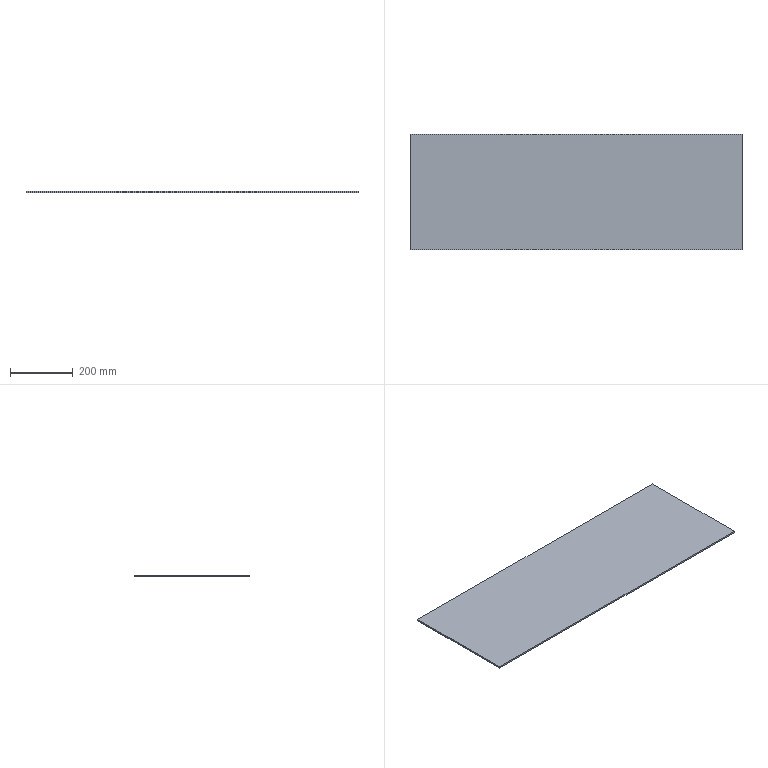Part | STEP file | JZHM | 1 solid | 6 faces | box 1060 x 370 x 5 mm | volume 1961000 mm3 | plane 6
STEP:
#1=CARTESIAN_POINT('',(0.,0.,0.));
#2=DIRECTION('',(0.,0.,1.));
#3=DIRECTION('',(1.,0.,0.));
#4=AXIS2_PLACEMENT_3D('',#1,#2,#3);
#5=CARTESIAN_POINT('',(-530.,185.,0.));
#6=VERTEX_POINT('',#5);
#7=CARTESIAN_POINT('',(-530.,-185.,0.));
#8=VERTEX_POINT('',#7);
#9=CARTESIAN_POINT('',(-530.,185.,0.));
#10=DIRECTION('',(0.,-1.,0.));
#11=VECTOR('',#10,1.);
#12=LINE('',#9,#11);
#13=CARTESIAN_POINT('',(-530.,185.,5.));
#14=DIRECTION('',(1.,0.,0.));
#15=DIRECTION('',(0.,0.,-1.));
#16=AXIS2_PLACEMENT_3D('',#13,#14,#15);
#17=PLANE('',#16);
#18=CARTESIAN_POINT('',(5.,0.));
#19=DIRECTION('',(0.,-1.));
#20=VECTOR('',#19,1.);
#21=LINE('',#18,#20);
#22=(GEOMETRIC_REPRESENTATION_CONTEXT(2)PARAMETRIC_REPRESENTATION_CONTEXT()REPRESENTATION_CONTEXT('',''));
#23=DEFINITIONAL_REPRESENTATION('',(#21),#22);
#24=PCURVE('',#17,#23);
#25=CARTESIAN_POINT('',(-530.,-185.,0.));
#26=DIRECTION('',(0.,0.,1.));
#27=DIRECTION('',(1.,0.,0.));
#28=AXIS2_PLACEMENT_3D('',#25,#26,#27);
#29=PLANE('',#28);
#30=CARTESIAN_POINT('',(0.,370.));
#31=DIRECTION('',(0.,-1.));
#32=VECTOR('',#31,1.);
#33=LINE('',#30,#32);
#34=(GEOMETRIC_REPRESENTATION_CONTEXT(2)PARAMETRIC_REPRESENTATION_CONTEXT()REPRESENTATION_CONTEXT('',''));
#35=DEFINITIONAL_REPRESENTATION('',(#33),#34);
#36=PCURVE('',#29,#35);
#37=SURFACE_CURVE('',#12,(#24,#36),.PCURVE_S1.);
#38=EDGE_CURVE('',#6,#8,#37,.T.);
#39=ORIENTED_EDGE('',*,*,#38,.T.);
#40=CARTESIAN_POINT('',(-530.,-185.,5.));
#41=VERTEX_POINT('',#40);
#42=CARTESIAN_POINT('',(-530.,-185.,5.));
#43=DIRECTION('',(0.,0.,-1.));
#44=VECTOR('',#43,1.);
#45=LINE('',#42,#44);
#46=CARTESIAN_POINT('',(0.,-370.));
#47=DIRECTION('',(1.,0.));
#48=VECTOR('',#47,1.);
#49=LINE('',#46,#48);
#50=(GEOMETRIC_REPRESENTATION_CONTEXT(2)PARAMETRIC_REPRESENTATION_CONTEXT()REPRESENTATION_CONTEXT('',''));
#51=DEFINITIONAL_REPRESENTATION('',(#49),#50);
#52=PCURVE('',#17,#51);
#53=CARTESIAN_POINT('',(-530.,-185.,5.));
#54=DIRECTION('',(0.,1.,0.));
#55=DIRECTION('',(0.,0.,1.));
#56=AXIS2_PLACEMENT_3D('',#53,#54,#55);
#57=PLANE('',#56);
#58=CARTESIAN_POINT('',(0.,0.));
#59=DIRECTION('',(-1.,0.));
#60=VECTOR('',#59,1.);
#61=LINE('',#58,#60);
#62=(GEOMETRIC_REPRESENTATION_CONTEXT(2)PARAMETRIC_REPRESENTATION_CONTEXT()REPRESENTATION_CONTEXT('',''));
#63=DEFINITIONAL_REPRESENTATION('',(#61),#62);
#64=PCURVE('',#57,#63);
#65=SURFACE_CURVE('',#45,(#52,#64),.PCURVE_S1.);
#66=EDGE_CURVE('',#41,#8,#65,.T.);
#67=ORIENTED_EDGE('',*,*,#66,.F.);
#68=CARTESIAN_POINT('',(-530.,185.,5.));
#69=VERTEX_POINT('',#68);
#70=CARTESIAN_POINT('',(-530.,185.,5.));
#71=DIRECTION('',(0.,-1.,0.));
#72=VECTOR('',#71,1.);
#73=LINE('',#70,#72);
#74=CARTESIAN_POINT('',(0.,0.));
#75=DIRECTION('',(0.,-1.));
#76=VECTOR('',#75,1.);
#77=LINE('',#74,#76);
#78=(GEOMETRIC_REPRESENTATION_CONTEXT(2)PARAMETRIC_REPRESENTATION_CONTEXT()REPRESENTATION_CONTEXT('',''));
#79=DEFINITIONAL_REPRESENTATION('',(#77),#78);
#80=PCURVE('',#17,#79);
#81=CARTESIAN_POINT('',(-530.,-185.,5.));
#82=DIRECTION('',(0.,0.,1.));
#83=DIRECTION('',(1.,0.,0.));
#84=AXIS2_PLACEMENT_3D('',#81,#82,#83);
#85=PLANE('',#84);
#86=CARTESIAN_POINT('',(0.,370.));
#87=DIRECTION('',(0.,-1.));
#88=VECTOR('',#87,1.);
#89=LINE('',#86,#88);
#90=(GEOMETRIC_REPRESENTATION_CONTEXT(2)PARAMETRIC_REPRESENTATION_CONTEXT()REPRESENTATION_CONTEXT('',''));
#91=DEFINITIONAL_REPRESENTATION('',(#89),#90);
#92=PCURVE('',#85,#91);
#93=SURFACE_CURVE('',#73,(#80,#92),.PCURVE_S1.);
#94=EDGE_CURVE('',#69,#41,#93,.T.);
#95=ORIENTED_EDGE('',*,*,#94,.F.);
#96=CARTESIAN_POINT('',(-530.,185.,5.));
#97=DIRECTION('',(0.,0.,-1.));
#98=VECTOR('',#97,1.);
#99=LINE('',#96,#98);
#100=CARTESIAN_POINT('',(0.,0.));
#101=DIRECTION('',(1.,0.));
#102=VECTOR('',#101,1.);
#103=LINE('',#100,#102);
#104=(GEOMETRIC_REPRESENTATION_CONTEXT(2)PARAMETRIC_REPRESENTATION_CONTEXT()REPRESENTATION_CONTEXT('',''));
#105=DEFINITIONAL_REPRESENTATION('',(#103),#104);
#106=PCURVE('',#17,#105);
#107=CARTESIAN_POINT('',(-530.,185.,5.));
#108=DIRECTION('',(0.,-1.,0.));
#109=DIRECTION('',(0.,0.,-1.));
#110=AXIS2_PLACEMENT_3D('',#107,#108,#109);
#111=PLANE('',#110);
#112=CARTESIAN_POINT('',(0.,0.));
#113=DIRECTION('',(1.,0.));
#114=VECTOR('',#113,1.);
#115=LINE('',#112,#114);
#116=(GEOMETRIC_REPRESENTATION_CONTEXT(2)PARAMETRIC_REPRESENTATION_CONTEXT()REPRESENTATION_CONTEXT('',''));
#117=DEFINITIONAL_REPRESENTATION('',(#115),#116);
#118=PCURVE('',#111,#117);
#119=SURFACE_CURVE('',#99,(#106,#118),.PCURVE_S1.);
#120=EDGE_CURVE('',#69,#6,#119,.T.);
#121=ORIENTED_EDGE('',*,*,#120,.T.);
#122=EDGE_LOOP('',(#39,#67,#95,#121));
#123=FACE_BOUND('',#122,.T.);
#124=ADVANCED_FACE('',(#123),#17,.F.);
#125=CARTESIAN_POINT('',(530.,-185.,0.));
#126=VERTEX_POINT('',#125);
#127=CARTESIAN_POINT('',(-530.,-185.,0.));
#128=DIRECTION('',(1.,0.,0.));
#129=VECTOR('',#128,1.);
#130=LINE('',#127,#129);
#131=CARTESIAN_POINT('',(-5.,0.));
#132=DIRECTION('',(0.,1.));
#133=VECTOR('',#132,1.);
#134=LINE('',#131,#133);
#135=(GEOMETRIC_REPRESENTATION_CONTEXT(2)PARAMETRIC_REPRESENTATION_CONTEXT()REPRESENTATION_CONTEXT('',''));
#136=DEFINITIONAL_REPRESENTATION('',(#134),#135);
#137=PCURVE('',#57,#136);
#138=CARTESIAN_POINT('',(0.,0.));
#139=DIRECTION('',(1.,0.));
#140=VECTOR('',#139,1.);
#141=LINE('',#138,#140);
#142=(GEOMETRIC_REPRESENTATION_CONTEXT(2)PARAMETRIC_REPRESENTATION_CONTEXT()REPRESENTATION_CONTEXT('',''));
#143=DEFINITIONAL_REPRESENTATION('',(#141),#142);
#144=PCURVE('',#29,#143);
#145=SURFACE_CURVE('',#130,(#137,#144),.PCURVE_S1.);
#146=EDGE_CURVE('',#8,#126,#145,.T.);
#147=ORIENTED_EDGE('',*,*,#146,.T.);
#148=CARTESIAN_POINT('',(530.,-185.,5.));
#149=VERTEX_POINT('',#148);
#150=CARTESIAN_POINT('',(530.,-185.,5.));
#151=DIRECTION('',(0.,0.,-1.));
#152=VECTOR('',#151,1.);
#153=LINE('',#150,#152);
#154=CARTESIAN_POINT('',(0.,1060.));
#155=DIRECTION('',(-1.,0.));
#156=VECTOR('',#155,1.);
#157=LINE('',#154,#156);
#158=(GEOMETRIC_REPRESENTATION_CONTEXT(2)PARAMETRIC_REPRESENTATION_CONTEXT()REPRESENTATION_CONTEXT('',''));
#159=DEFINITIONAL_REPRESENTATION('',(#157),#158);
#160=PCURVE('',#57,#159);
#161=CARTESIAN_POINT('',(530.,185.,5.));
#162=DIRECTION('',(-1.,0.,0.));
#163=DIRECTION('',(0.,0.,1.));
#164=AXIS2_PLACEMENT_3D('',#161,#162,#163);
#165=PLANE('',#164);
#166=CARTESIAN_POINT('',(0.,-370.));
#167=DIRECTION('',(-1.,0.));
#168=VECTOR('',#167,1.);
#169=LINE('',#166,#168);
#170=(GEOMETRIC_REPRESENTATION_CONTEXT(2)PARAMETRIC_REPRESENTATION_CONTEXT()REPRESENTATION_CONTEXT('',''));
#171=DEFINITIONAL_REPRESENTATION('',(#169),#170);
#172=PCURVE('',#165,#171);
#173=SURFACE_CURVE('',#153,(#160,#172),.PCURVE_S1.);
#174=EDGE_CURVE('',#149,#126,#173,.T.);
#175=ORIENTED_EDGE('',*,*,#174,.F.);
#176=CARTESIAN_POINT('',(-530.,-185.,5.));
#177=DIRECTION('',(1.,0.,0.));
#178=VECTOR('',#177,1.);
#179=LINE('',#176,#178);
#180=CARTESIAN_POINT('',(0.,0.));
#181=DIRECTION('',(0.,1.));
#182=VECTOR('',#181,1.);
#183=LINE('',#180,#182);
#184=(GEOMETRIC_REPRESENTATION_CONTEXT(2)PARAMETRIC_REPRESENTATION_CONTEXT()REPRESENTATION_CONTEXT('',''));
#185=DEFINITIONAL_REPRESENTATION('',(#183),#184);
#186=PCURVE('',#57,#185);
#187=CARTESIAN_POINT('',(0.,0.));
#188=DIRECTION('',(1.,0.));
#189=VECTOR('',#188,1.);
#190=LINE('',#187,#189);
#191=(GEOMETRIC_REPRESENTATION_CONTEXT(2)PARAMETRIC_REPRESENTATION_CONTEXT()REPRESENTATION_CONTEXT('',''));
#192=DEFINITIONAL_REPRESENTATION('',(#190),#191);
#193=PCURVE('',#85,#192);
#194=SURFACE_CURVE('',#179,(#186,#193),.PCURVE_S1.);
#195=EDGE_CURVE('',#41,#149,#194,.T.);
#196=ORIENTED_EDGE('',*,*,#195,.F.);
#197=ORIENTED_EDGE('',*,*,#66,.T.);
#198=EDGE_LOOP('',(#147,#175,#196,#197));
#199=FACE_BOUND('',#198,.T.);
#200=ADVANCED_FACE('',(#199),#57,.F.);
#201=CARTESIAN_POINT('',(530.,185.,0.));
#202=VERTEX_POINT('',#201);
#203=CARTESIAN_POINT('',(530.,185.,0.));
#204=DIRECTION('',(0.,1.,0.));
#205=VECTOR('',#204,1.);
#206=LINE('',#203,#205);
#207=CARTESIAN_POINT('',(-5.,0.));
#208=DIRECTION('',(0.,1.));
#209=VECTOR('',#208,1.);
#210=LINE('',#207,#209);
#211=(GEOMETRIC_REPRESENTATION_CONTEXT(2)PARAMETRIC_REPRESENTATION_CONTEXT()REPRESENTATION_CONTEXT('',''));
#212=DEFINITIONAL_REPRESENTATION('',(#210),#211);
#213=PCURVE('',#165,#212);
#214=CARTESIAN_POINT('',(1060.,370.));
#215=DIRECTION('',(0.,1.));
#216=VECTOR('',#215,1.);
#217=LINE('',#214,#216);
#218=(GEOMETRIC_REPRESENTATION_CONTEXT(2)PARAMETRIC_REPRESENTATION_CONTEXT()REPRESENTATION_CONTEXT('',''));
#219=DEFINITIONAL_REPRESENTATION('',(#217),#218);
#220=PCURVE('',#29,#219);
#221=SURFACE_CURVE('',#206,(#213,#220),.PCURVE_S1.);
#222=EDGE_CURVE('',#126,#202,#221,.T.);
#223=ORIENTED_EDGE('',*,*,#222,.T.);
#224=CARTESIAN_POINT('',(530.,185.,5.));
#225=VERTEX_POINT('',#224);
#226=CARTESIAN_POINT('',(530.,185.,5.));
#227=DIRECTION('',(0.,0.,-1.));
#228=VECTOR('',#227,1.);
#229=LINE('',#226,#228);
#230=CARTESIAN_POINT('',(0.,0.));
#231=DIRECTION('',(-1.,0.));
#232=VECTOR('',#231,1.);
#233=LINE('',#230,#232);
#234=(GEOMETRIC_REPRESENTATION_CONTEXT(2)PARAMETRIC_REPRESENTATION_CONTEXT()REPRESENTATION_CONTEXT('',''));
#235=DEFINITIONAL_REPRESENTATION('',(#233),#234);
#236=PCURVE('',#165,#235);
#237=CARTESIAN_POINT('',(0.,1060.));
#238=DIRECTION('',(1.,0.));
#239=VECTOR('',#238,1.);
#240=LINE('',#237,#239);
#241=(GEOMETRIC_REPRESENTATION_CONTEXT(2)PARAMETRIC_REPRESENTATION_CONTEXT()REPRESENTATION_CONTEXT('',''));
#242=DEFINITIONAL_REPRESENTATION('',(#240),#241);
#243=PCURVE('',#111,#242);
#244=SURFACE_CURVE('',#229,(#236,#243),.PCURVE_S1.);
#245=EDGE_CURVE('',#225,#202,#244,.T.);
#246=ORIENTED_EDGE('',*,*,#245,.F.);
#247=CARTESIAN_POINT('',(530.,185.,5.));
#248=DIRECTION('',(0.,1.,0.));
#249=VECTOR('',#248,1.);
#250=LINE('',#247,#249);
#251=CARTESIAN_POINT('',(0.,0.));
#252=DIRECTION('',(0.,1.));
#253=VECTOR('',#252,1.);
#254=LINE('',#251,#253);
#255=(GEOMETRIC_REPRESENTATION_CONTEXT(2)PARAMETRIC_REPRESENTATION_CONTEXT()REPRESENTATION_CONTEXT('',''));
#256=DEFINITIONAL_REPRESENTATION('',(#254),#255);
#257=PCURVE('',#165,#256);
#258=CARTESIAN_POINT('',(1060.,370.));
#259=DIRECTION('',(0.,1.));
#260=VECTOR('',#259,1.);
#261=LINE('',#258,#260);
#262=(GEOMETRIC_REPRESENTATION_CONTEXT(2)PARAMETRIC_REPRESENTATION_CONTEXT()REPRESENTATION_CONTEXT('',''));
#263=DEFINITIONAL_REPRESENTATION('',(#261),#262);
#264=PCURVE('',#85,#263);
#265=SURFACE_CURVE('',#250,(#257,#264),.PCURVE_S1.);
#266=EDGE_CURVE('',#149,#225,#265,.T.);
#267=ORIENTED_EDGE('',*,*,#266,.F.);
#268=ORIENTED_EDGE('',*,*,#174,.T.);
#269=EDGE_LOOP('',(#223,#246,#267,#268));
#270=FACE_BOUND('',#269,.T.);
#271=ADVANCED_FACE('',(#270),#165,.F.);
#272=CARTESIAN_POINT('',(-530.,185.,0.));
#273=DIRECTION('',(-1.,0.,0.));
#274=VECTOR('',#273,1.);
#275=LINE('',#272,#274);
#276=CARTESIAN_POINT('',(5.,0.));
#277=DIRECTION('',(0.,-1.));
#278=VECTOR('',#277,1.);
#279=LINE('',#276,#278);
#280=(GEOMETRIC_REPRESENTATION_CONTEXT(2)PARAMETRIC_REPRESENTATION_CONTEXT()REPRESENTATION_CONTEXT('',''));
#281=DEFINITIONAL_REPRESENTATION('',(#279),#280);
#282=PCURVE('',#111,#281);
#283=CARTESIAN_POINT('',(0.,370.));
#284=DIRECTION('',(-1.,0.));
#285=VECTOR('',#284,1.);
#286=LINE('',#283,#285);
#287=(GEOMETRIC_REPRESENTATION_CONTEXT(2)PARAMETRIC_REPRESENTATION_CONTEXT()REPRESENTATION_CONTEXT('',''));
#288=DEFINITIONAL_REPRESENTATION('',(#286),#287);
#289=PCURVE('',#29,#288);
#290=SURFACE_CURVE('',#275,(#282,#289),.PCURVE_S1.);
#291=EDGE_CURVE('',#202,#6,#290,.T.);
#292=ORIENTED_EDGE('',*,*,#291,.T.);
#293=ORIENTED_EDGE('',*,*,#120,.F.);
#294=CARTESIAN_POINT('',(-530.,185.,5.));
#295=DIRECTION('',(-1.,0.,0.));
#296=VECTOR('',#295,1.);
#297=LINE('',#294,#296);
#298=CARTESIAN_POINT('',(0.,0.));
#299=DIRECTION('',(0.,-1.));
#300=VECTOR('',#299,1.);
#301=LINE('',#298,#300);
#302=(GEOMETRIC_REPRESENTATION_CONTEXT(2)PARAMETRIC_REPRESENTATION_CONTEXT()REPRESENTATION_CONTEXT('',''));
#303=DEFINITIONAL_REPRESENTATION('',(#301),#302);
#304=PCURVE('',#111,#303);
#305=CARTESIAN_POINT('',(0.,370.));
#306=DIRECTION('',(-1.,0.));
#307=VECTOR('',#306,1.);
#308=LINE('',#305,#307);
#309=(GEOMETRIC_REPRESENTATION_CONTEXT(2)PARAMETRIC_REPRESENTATION_CONTEXT()REPRESENTATION_CONTEXT('',''));
#310=DEFINITIONAL_REPRESENTATION('',(#308),#309);
#311=PCURVE('',#85,#310);
#312=SURFACE_CURVE('',#297,(#304,#311),.PCURVE_S1.);
#313=EDGE_CURVE('',#225,#69,#312,.T.);
#314=ORIENTED_EDGE('',*,*,#313,.F.);
#315=ORIENTED_EDGE('',*,*,#245,.T.);
#316=EDGE_LOOP('',(#292,#293,#314,#315));
#317=FACE_BOUND('',#316,.T.);
#318=ADVANCED_FACE('',(#317),#111,.F.);
#319=ORIENTED_EDGE('',*,*,#94,.T.);
#320=ORIENTED_EDGE('',*,*,#195,.T.);
#321=ORIENTED_EDGE('',*,*,#266,.T.);
#322=ORIENTED_EDGE('',*,*,#313,.T.);
#323=EDGE_LOOP('',(#319,#320,#321,#322));
#324=FACE_BOUND('',#323,.T.);
#325=ADVANCED_FACE('',(#324),#85,.T.);
#326=ORIENTED_EDGE('',*,*,#38,.F.);
#327=ORIENTED_EDGE('',*,*,#291,.F.);
#328=ORIENTED_EDGE('',*,*,#222,.F.);
#329=ORIENTED_EDGE('',*,*,#146,.F.);
#330=EDGE_LOOP('',(#326,#327,#328,#329));
#331=FACE_BOUND('',#330,.T.);
#332=ADVANCED_FACE('',(#331),#29,.F.);
#333=CLOSED_SHELL('',(#124,#200,#271,#318,#325,#332));
#334=MANIFOLD_SOLID_BREP('',#333);
#335=(LENGTH_UNIT()NAMED_UNIT(*)SI_UNIT(.MILLI.,.METRE.));
#336=UNCERTAINTY_MEASURE_WITH_UNIT(LENGTH_MEASURE(0.0000001),#335,'','');
#337=(NAMED_UNIT(*)PLANE_ANGLE_UNIT()SI_UNIT($,.RADIAN.));
#338=(NAMED_UNIT(*)SI_UNIT($,.STERADIAN.)SOLID_ANGLE_UNIT());
#339=(GEOMETRIC_REPRESENTATION_CONTEXT(3)GLOBAL_UNCERTAINTY_ASSIGNED_CONTEXT((#336))GLOBAL_UNIT_ASSIGNED_CONTEXT((#335,#337,#338))REPRESENTATION_CONTEXT('',''));
#340=ADVANCED_BREP_SHAPE_REPRESENTATION('',(#4,#334),#339);